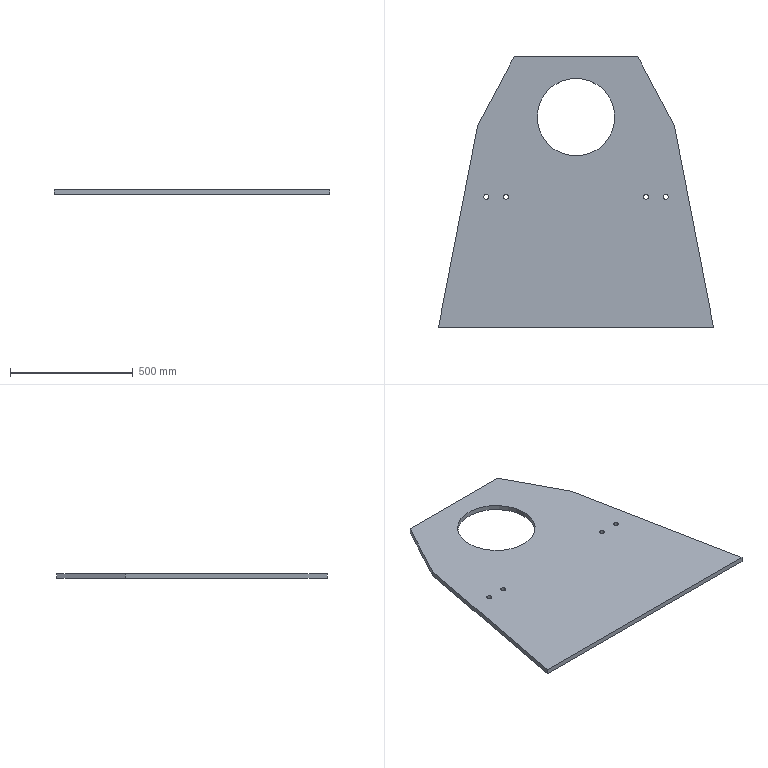Part | SolidWorks | features BaseBody 1 | 1 solid | 18 faces | box 1120 x 1100 x 20 mm | volume 17817233 mm3 | cylinder 10 | plane 8 | commonest cylinder face diameters 20 x8 316 x2
STEP:
#1=CARTESIAN_POINT('',(4376.449,1438.717,20.));
#2=VERTEX_POINT('',#1);
#3=CARTESIAN_POINT('',(4396.449,1438.717,20.));
#4=VERTEX_POINT('',#3);
#5=CARTESIAN_POINT('',(4386.449,1438.717,20.));
#6=DIRECTION('',(0.,0.,1.));
#7=DIRECTION('',(1.,0.,0.));
#8=AXIS2_PLACEMENT_3D('',#5,#6,#7);
#9=CIRCLE('',#8,10.);
#10=EDGE_CURVE('',#2,#4,#9,.T.);
#11=ORIENTED_EDGE('',*,*,#10,.T.);
#12=CARTESIAN_POINT('',(4396.449,1438.717,0.));
#13=VERTEX_POINT('',#12);
#14=CARTESIAN_POINT('',(4396.449,1438.717,20.));
#15=DIRECTION('',(0.,0.,-1.));
#16=VECTOR('',#15,1000.);
#17=LINE('',#14,#16);
#18=EDGE_CURVE('',#4,#13,#17,.T.);
#19=ORIENTED_EDGE('',*,*,#18,.T.);
#20=CARTESIAN_POINT('',(4376.449,1438.717,0.));
#21=VERTEX_POINT('',#20);
#22=CARTESIAN_POINT('',(4386.449,1438.717,0.));
#23=DIRECTION('',(0.,0.,1.));
#24=DIRECTION('',(1.,0.,0.));
#25=AXIS2_PLACEMENT_3D('',#22,#23,#24);
#26=CIRCLE('',#25,10.);
#27=EDGE_CURVE('',#21,#13,#26,.T.);
#28=ORIENTED_EDGE('',*,*,#27,.F.);
#29=CARTESIAN_POINT('',(4376.449,1438.717,20.));
#30=DIRECTION('',(0.,0.,-1.));
#31=VECTOR('',#30,1000.);
#32=LINE('',#29,#31);
#33=EDGE_CURVE('',#2,#21,#32,.T.);
#34=ORIENTED_EDGE('',*,*,#33,.F.);
#35=EDGE_LOOP('',(#11,#19,#28,#34));
#36=FACE_OUTER_BOUND('',#35,.T.);
#37=CARTESIAN_POINT('',(4386.449,1438.717,20.));
#38=DIRECTION('',(0.,0.,-1.));
#39=DIRECTION('',(-1.,0.,0.));
#40=AXIS2_PLACEMENT_3D('',#37,#38,#39);
#41=CYLINDRICAL_SURFACE('',#40,10.);
#42=ADVANCED_FACE('',(#36),#41,.F.);
#43=CARTESIAN_POINT('',(4456.449,1438.717,20.));
#44=VERTEX_POINT('',#43);
#45=CARTESIAN_POINT('',(4476.449,1438.717,20.));
#46=VERTEX_POINT('',#45);
#47=CARTESIAN_POINT('',(4466.449,1438.717,20.));
#48=DIRECTION('',(0.,0.,1.));
#49=DIRECTION('',(1.,0.,0.));
#50=AXIS2_PLACEMENT_3D('',#47,#48,#49);
#51=CIRCLE('',#50,10.);
#52=EDGE_CURVE('',#44,#46,#51,.T.);
#53=ORIENTED_EDGE('',*,*,#52,.T.);
#54=CARTESIAN_POINT('',(4476.449,1438.717,0.));
#55=VERTEX_POINT('',#54);
#56=CARTESIAN_POINT('',(4476.449,1438.717,20.));
#57=DIRECTION('',(0.,0.,-1.));
#58=VECTOR('',#57,1000.);
#59=LINE('',#56,#58);
#60=EDGE_CURVE('',#46,#55,#59,.T.);
#61=ORIENTED_EDGE('',*,*,#60,.T.);
#62=CARTESIAN_POINT('',(4456.449,1438.717,0.));
#63=VERTEX_POINT('',#62);
#64=CARTESIAN_POINT('',(4466.449,1438.717,0.));
#65=DIRECTION('',(0.,0.,1.));
#66=DIRECTION('',(1.,0.,0.));
#67=AXIS2_PLACEMENT_3D('',#64,#65,#66);
#68=CIRCLE('',#67,10.);
#69=EDGE_CURVE('',#63,#55,#68,.T.);
#70=ORIENTED_EDGE('',*,*,#69,.F.);
#71=CARTESIAN_POINT('',(4456.449,1438.717,20.));
#72=DIRECTION('',(0.,0.,-1.));
#73=VECTOR('',#72,1000.);
#74=LINE('',#71,#73);
#75=EDGE_CURVE('',#44,#63,#74,.T.);
#76=ORIENTED_EDGE('',*,*,#75,.F.);
#77=EDGE_LOOP('',(#53,#61,#70,#76));
#78=FACE_OUTER_BOUND('',#77,.T.);
#79=CARTESIAN_POINT('',(4466.449,1438.717,20.));
#80=DIRECTION('',(0.,0.,-1.));
#81=DIRECTION('',(-1.,0.,0.));
#82=AXIS2_PLACEMENT_3D('',#79,#80,#81);
#83=CYLINDRICAL_SURFACE('',#82,10.);
#84=ADVANCED_FACE('',(#78),#83,.F.);
#85=CARTESIAN_POINT('',(4593.449,1763.717,20.));
#86=VERTEX_POINT('',#85);
#87=CARTESIAN_POINT('',(4909.449,1763.717,20.));
#88=VERTEX_POINT('',#87);
#89=CARTESIAN_POINT('',(4751.449,1763.717,20.));
#90=DIRECTION('',(0.,0.,1.));
#91=DIRECTION('',(1.,0.,0.));
#92=AXIS2_PLACEMENT_3D('',#89,#90,#91);
#93=CIRCLE('',#92,158.);
#94=EDGE_CURVE('',#86,#88,#93,.T.);
#95=ORIENTED_EDGE('',*,*,#94,.T.);
#96=CARTESIAN_POINT('',(4909.449,1763.717,0.));
#97=VERTEX_POINT('',#96);
#98=CARTESIAN_POINT('',(4909.449,1763.717,20.));
#99=DIRECTION('',(0.,0.,-1.));
#100=VECTOR('',#99,1000.);
#101=LINE('',#98,#100);
#102=EDGE_CURVE('',#88,#97,#101,.T.);
#103=ORIENTED_EDGE('',*,*,#102,.T.);
#104=CARTESIAN_POINT('',(4593.449,1763.717,0.));
#105=VERTEX_POINT('',#104);
#106=CARTESIAN_POINT('',(4751.449,1763.717,0.));
#107=DIRECTION('',(0.,0.,1.));
#108=DIRECTION('',(1.,0.,0.));
#109=AXIS2_PLACEMENT_3D('',#106,#107,#108);
#110=CIRCLE('',#109,158.);
#111=EDGE_CURVE('',#105,#97,#110,.T.);
#112=ORIENTED_EDGE('',*,*,#111,.F.);
#113=CARTESIAN_POINT('',(4593.449,1763.717,20.));
#114=DIRECTION('',(0.,0.,-1.));
#115=VECTOR('',#114,1000.);
#116=LINE('',#113,#115);
#117=EDGE_CURVE('',#86,#105,#116,.T.);
#118=ORIENTED_EDGE('',*,*,#117,.F.);
#119=EDGE_LOOP('',(#95,#103,#112,#118));
#120=FACE_OUTER_BOUND('',#119,.T.);
#121=CARTESIAN_POINT('',(4751.449,1763.717,20.));
#122=DIRECTION('',(0.,0.,-1.));
#123=DIRECTION('',(-1.,0.,0.));
#124=AXIS2_PLACEMENT_3D('',#121,#122,#123);
#125=CYLINDRICAL_SURFACE('',#124,158.);
#126=ADVANCED_FACE('',(#120),#125,.F.);
#127=CARTESIAN_POINT('',(5106.449,1438.717,20.));
#128=VERTEX_POINT('',#127);
#129=CARTESIAN_POINT('',(5126.449,1438.717,20.));
#130=VERTEX_POINT('',#129);
#131=CARTESIAN_POINT('',(5116.449,1438.717,20.));
#132=DIRECTION('',(0.,0.,1.));
#133=DIRECTION('',(1.,0.,0.));
#134=AXIS2_PLACEMENT_3D('',#131,#132,#133);
#135=CIRCLE('',#134,10.);
#136=EDGE_CURVE('',#128,#130,#135,.T.);
#137=ORIENTED_EDGE('',*,*,#136,.T.);
#138=CARTESIAN_POINT('',(5126.449,1438.717,0.));
#139=VERTEX_POINT('',#138);
#140=CARTESIAN_POINT('',(5126.449,1438.717,20.));
#141=DIRECTION('',(0.,0.,-1.));
#142=VECTOR('',#141,1000.);
#143=LINE('',#140,#142);
#144=EDGE_CURVE('',#130,#139,#143,.T.);
#145=ORIENTED_EDGE('',*,*,#144,.T.);
#146=CARTESIAN_POINT('',(5106.449,1438.717,0.));
#147=VERTEX_POINT('',#146);
#148=CARTESIAN_POINT('',(5116.449,1438.717,0.));
#149=DIRECTION('',(0.,0.,1.));
#150=DIRECTION('',(1.,0.,0.));
#151=AXIS2_PLACEMENT_3D('',#148,#149,#150);
#152=CIRCLE('',#151,10.);
#153=EDGE_CURVE('',#147,#139,#152,.T.);
#154=ORIENTED_EDGE('',*,*,#153,.F.);
#155=CARTESIAN_POINT('',(5106.449,1438.717,20.));
#156=DIRECTION('',(0.,0.,-1.));
#157=VECTOR('',#156,1000.);
#158=LINE('',#155,#157);
#159=EDGE_CURVE('',#128,#147,#158,.T.);
#160=ORIENTED_EDGE('',*,*,#159,.F.);
#161=EDGE_LOOP('',(#137,#145,#154,#160));
#162=FACE_OUTER_BOUND('',#161,.T.);
#163=CARTESIAN_POINT('',(5116.449,1438.717,20.));
#164=DIRECTION('',(0.,0.,-1.));
#165=DIRECTION('',(-1.,0.,0.));
#166=AXIS2_PLACEMENT_3D('',#163,#164,#165);
#167=CYLINDRICAL_SURFACE('',#166,10.);
#168=ADVANCED_FACE('',(#162),#167,.F.);
#169=CARTESIAN_POINT('',(5026.449,1438.717,20.));
#170=VERTEX_POINT('',#169);
#171=CARTESIAN_POINT('',(5046.449,1438.717,20.));
#172=VERTEX_POINT('',#171);
#173=CARTESIAN_POINT('',(5036.449,1438.717,20.));
#174=DIRECTION('',(0.,0.,1.));
#175=DIRECTION('',(1.,0.,0.));
#176=AXIS2_PLACEMENT_3D('',#173,#174,#175);
#177=CIRCLE('',#176,10.);
#178=EDGE_CURVE('',#170,#172,#177,.T.);
#179=ORIENTED_EDGE('',*,*,#178,.T.);
#180=CARTESIAN_POINT('',(5046.449,1438.717,0.));
#181=VERTEX_POINT('',#180);
#182=CARTESIAN_POINT('',(5046.449,1438.717,20.));
#183=DIRECTION('',(0.,0.,-1.));
#184=VECTOR('',#183,1000.);
#185=LINE('',#182,#184);
#186=EDGE_CURVE('',#172,#181,#185,.T.);
#187=ORIENTED_EDGE('',*,*,#186,.T.);
#188=CARTESIAN_POINT('',(5026.449,1438.717,0.));
#189=VERTEX_POINT('',#188);
#190=CARTESIAN_POINT('',(5036.449,1438.717,0.));
#191=DIRECTION('',(0.,0.,1.));
#192=DIRECTION('',(1.,0.,0.));
#193=AXIS2_PLACEMENT_3D('',#190,#191,#192);
#194=CIRCLE('',#193,10.);
#195=EDGE_CURVE('',#189,#181,#194,.T.);
#196=ORIENTED_EDGE('',*,*,#195,.F.);
#197=CARTESIAN_POINT('',(5026.449,1438.717,20.));
#198=DIRECTION('',(0.,0.,-1.));
#199=VECTOR('',#198,1000.);
#200=LINE('',#197,#199);
#201=EDGE_CURVE('',#170,#189,#200,.T.);
#202=ORIENTED_EDGE('',*,*,#201,.F.);
#203=EDGE_LOOP('',(#179,#187,#196,#202));
#204=FACE_OUTER_BOUND('',#203,.T.);
#205=CARTESIAN_POINT('',(5036.449,1438.717,20.));
#206=DIRECTION('',(0.,0.,-1.));
#207=DIRECTION('',(-1.,0.,0.));
#208=AXIS2_PLACEMENT_3D('',#205,#206,#207);
#209=CYLINDRICAL_SURFACE('',#208,10.);
#210=ADVANCED_FACE('',(#204),#209,.F.);
#211=ORIENTED_EDGE('',*,*,#52,.F.);
#212=CARTESIAN_POINT('',(4466.449,1438.717,20.));
#213=DIRECTION('',(0.,0.,1.));
#214=DIRECTION('',(1.,0.,0.));
#215=AXIS2_PLACEMENT_3D('',#212,#213,#214);
#216=CIRCLE('',#215,10.);
#217=EDGE_CURVE('',#46,#44,#216,.T.);
#218=ORIENTED_EDGE('',*,*,#217,.F.);
#219=EDGE_LOOP('',(#211,#218));
#220=FACE_BOUND('',#219,.T.);
#221=ORIENTED_EDGE('',*,*,#136,.F.);
#222=CARTESIAN_POINT('',(5116.449,1438.717,20.));
#223=DIRECTION('',(0.,0.,1.));
#224=DIRECTION('',(1.,0.,0.));
#225=AXIS2_PLACEMENT_3D('',#222,#223,#224);
#226=CIRCLE('',#225,10.);
#227=EDGE_CURVE('',#130,#128,#226,.T.);
#228=ORIENTED_EDGE('',*,*,#227,.F.);
#229=EDGE_LOOP('',(#221,#228));
#230=FACE_BOUND('',#229,.T.);
#231=CARTESIAN_POINT('',(4351.039,1729.734,20.));
#232=VERTEX_POINT('',#231);
#233=CARTESIAN_POINT('',(4191.449,908.717,20.));
#234=VERTEX_POINT('',#233);
#235=CARTESIAN_POINT('',(4351.039,1729.734,20.));
#236=DIRECTION('',(-0.1908,-0.9816,0.));
#237=VECTOR('',#236,1000.);
#238=LINE('',#235,#237);
#239=EDGE_CURVE('',#232,#234,#238,.T.);
#240=ORIENTED_EDGE('',*,*,#239,.T.);
#241=CARTESIAN_POINT('',(5311.449,908.717,20.));
#242=VERTEX_POINT('',#241);
#243=CARTESIAN_POINT('',(4191.449,908.717,20.));
#244=DIRECTION('',(1.,0.,0.));
#245=VECTOR('',#244,1000.);
#246=LINE('',#243,#245);
#247=EDGE_CURVE('',#234,#242,#246,.T.);
#248=ORIENTED_EDGE('',*,*,#247,.T.);
#249=CARTESIAN_POINT('',(5151.86,1729.734,20.));
#250=VERTEX_POINT('',#249);
#251=CARTESIAN_POINT('',(5151.86,1729.734,20.));
#252=DIRECTION('',(-0.1908,0.9816,0.));
#253=VECTOR('',#252,1000.);
#254=LINE('',#251,#253);
#255=EDGE_CURVE('',#242,#250,#254,.T.);
#256=ORIENTED_EDGE('',*,*,#255,.T.);
#257=CARTESIAN_POINT('',(5003.522,2008.717,20.));
#258=VERTEX_POINT('',#257);
#259=CARTESIAN_POINT('',(5003.522,2008.717,20.));
#260=DIRECTION('',(-0.4695,0.8829,0.));
#261=VECTOR('',#260,1000.);
#262=LINE('',#259,#261);
#263=EDGE_CURVE('',#250,#258,#262,.T.);
#264=ORIENTED_EDGE('',*,*,#263,.T.);
#265=CARTESIAN_POINT('',(4499.377,2008.717,20.));
#266=VERTEX_POINT('',#265);
#267=CARTESIAN_POINT('',(4499.377,2008.717,20.));
#268=DIRECTION('',(-1.,0.,0.));
#269=VECTOR('',#268,1000.);
#270=LINE('',#267,#269);
#271=EDGE_CURVE('',#258,#266,#270,.T.);
#272=ORIENTED_EDGE('',*,*,#271,.T.);
#273=CARTESIAN_POINT('',(4499.377,2008.717,20.));
#274=DIRECTION('',(-0.4695,-0.8829,0.));
#275=VECTOR('',#274,1000.);
#276=LINE('',#273,#275);
#277=EDGE_CURVE('',#266,#232,#276,.T.);
#278=ORIENTED_EDGE('',*,*,#277,.T.);
#279=EDGE_LOOP('',(#240,#248,#256,#264,#272,#278));
#280=FACE_OUTER_BOUND('',#279,.T.);
#281=ORIENTED_EDGE('',*,*,#178,.F.);
#282=CARTESIAN_POINT('',(5036.449,1438.717,20.));
#283=DIRECTION('',(0.,0.,1.));
#284=DIRECTION('',(1.,0.,0.));
#285=AXIS2_PLACEMENT_3D('',#282,#283,#284);
#286=CIRCLE('',#285,10.);
#287=EDGE_CURVE('',#172,#170,#286,.T.);
#288=ORIENTED_EDGE('',*,*,#287,.F.);
#289=EDGE_LOOP('',(#281,#288));
#290=FACE_BOUND('',#289,.T.);
#291=ORIENTED_EDGE('',*,*,#94,.F.);
#292=CARTESIAN_POINT('',(4751.449,1763.717,20.));
#293=DIRECTION('',(0.,0.,1.));
#294=DIRECTION('',(1.,0.,0.));
#295=AXIS2_PLACEMENT_3D('',#292,#293,#294);
#296=CIRCLE('',#295,158.);
#297=EDGE_CURVE('',#88,#86,#296,.T.);
#298=ORIENTED_EDGE('',*,*,#297,.F.);
#299=EDGE_LOOP('',(#291,#298));
#300=FACE_BOUND('',#299,.T.);
#301=ORIENTED_EDGE('',*,*,#10,.F.);
#302=CARTESIAN_POINT('',(4386.449,1438.717,20.));
#303=DIRECTION('',(0.,0.,1.));
#304=DIRECTION('',(1.,0.,0.));
#305=AXIS2_PLACEMENT_3D('',#302,#303,#304);
#306=CIRCLE('',#305,10.);
#307=EDGE_CURVE('',#4,#2,#306,.T.);
#308=ORIENTED_EDGE('',*,*,#307,.F.);
#309=EDGE_LOOP('',(#301,#308));
#310=FACE_BOUND('',#309,.T.);
#311=CARTESIAN_POINT('',(0.,0.,20.));
#312=DIRECTION('',(0.,0.,1.));
#313=DIRECTION('',(1.,0.,0.));
#314=AXIS2_PLACEMENT_3D('',#311,#312,#313);
#315=PLANE('',#314);
#316=ADVANCED_FACE('',(#220,#230,#280,#290,#300,#310),#315,.T.);
#317=CARTESIAN_POINT('',(4351.039,1729.734,0.));
#318=VERTEX_POINT('',#317);
#319=CARTESIAN_POINT('',(4191.449,908.717,0.));
#320=VERTEX_POINT('',#319);
#321=CARTESIAN_POINT('',(4351.039,1729.734,0.));
#322=DIRECTION('',(-0.1908,-0.9816,0.));
#323=VECTOR('',#322,1000.);
#324=LINE('',#321,#323);
#325=EDGE_CURVE('',#318,#320,#324,.T.);
#326=ORIENTED_EDGE('',*,*,#325,.F.);
#327=CARTESIAN_POINT('',(4499.377,2008.717,0.));
#328=VERTEX_POINT('',#327);
#329=CARTESIAN_POINT('',(4499.377,2008.717,0.));
#330=DIRECTION('',(-0.4695,-0.8829,0.));
#331=VECTOR('',#330,1000.);
#332=LINE('',#329,#331);
#333=EDGE_CURVE('',#328,#318,#332,.T.);
#334=ORIENTED_EDGE('',*,*,#333,.F.);
#335=CARTESIAN_POINT('',(5003.522,2008.717,0.));
#336=VERTEX_POINT('',#335);
#337=CARTESIAN_POINT('',(4499.377,2008.717,0.));
#338=DIRECTION('',(-1.,0.,0.));
#339=VECTOR('',#338,1000.);
#340=LINE('',#337,#339);
#341=EDGE_CURVE('',#336,#328,#340,.T.);
#342=ORIENTED_EDGE('',*,*,#341,.F.);
#343=CARTESIAN_POINT('',(5151.86,1729.734,0.));
#344=VERTEX_POINT('',#343);
#345=CARTESIAN_POINT('',(5003.522,2008.717,0.));
#346=DIRECTION('',(-0.4695,0.8829,0.));
#347=VECTOR('',#346,1000.);
#348=LINE('',#345,#347);
#349=EDGE_CURVE('',#344,#336,#348,.T.);
#350=ORIENTED_EDGE('',*,*,#349,.F.);
#351=CARTESIAN_POINT('',(5311.449,908.717,0.));
#352=VERTEX_POINT('',#351);
#353=CARTESIAN_POINT('',(5151.86,1729.734,0.));
#354=DIRECTION('',(-0.1908,0.9816,0.));
#355=VECTOR('',#354,1000.);
#356=LINE('',#353,#355);
#357=EDGE_CURVE('',#352,#344,#356,.T.);
#358=ORIENTED_EDGE('',*,*,#357,.F.);
#359=CARTESIAN_POINT('',(4191.449,908.717,0.));
#360=DIRECTION('',(1.,0.,0.));
#361=VECTOR('',#360,1000.);
#362=LINE('',#359,#361);
#363=EDGE_CURVE('',#320,#352,#362,.T.);
#364=ORIENTED_EDGE('',*,*,#363,.F.);
#365=EDGE_LOOP('',(#326,#334,#342,#350,#358,#364));
#366=FACE_OUTER_BOUND('',#365,.T.);
#367=ORIENTED_EDGE('',*,*,#195,.T.);
#368=CARTESIAN_POINT('',(5036.449,1438.717,0.));
#369=DIRECTION('',(0.,0.,1.));
#370=DIRECTION('',(1.,0.,0.));
#371=AXIS2_PLACEMENT_3D('',#368,#369,#370);
#372=CIRCLE('',#371,10.);
#373=EDGE_CURVE('',#181,#189,#372,.T.);
#374=ORIENTED_EDGE('',*,*,#373,.T.);
#375=EDGE_LOOP('',(#367,#374));
#376=FACE_BOUND('',#375,.T.);
#377=ORIENTED_EDGE('',*,*,#153,.T.);
#378=CARTESIAN_POINT('',(5116.449,1438.717,0.));
#379=DIRECTION('',(0.,0.,1.));
#380=DIRECTION('',(1.,0.,0.));
#381=AXIS2_PLACEMENT_3D('',#378,#379,#380);
#382=CIRCLE('',#381,10.);
#383=EDGE_CURVE('',#139,#147,#382,.T.);
#384=ORIENTED_EDGE('',*,*,#383,.T.);
#385=EDGE_LOOP('',(#377,#384));
#386=FACE_BOUND('',#385,.T.);
#387=ORIENTED_EDGE('',*,*,#111,.T.);
#388=CARTESIAN_POINT('',(4751.449,1763.717,0.));
#389=DIRECTION('',(0.,0.,1.));
#390=DIRECTION('',(1.,0.,0.));
#391=AXIS2_PLACEMENT_3D('',#388,#389,#390);
#392=CIRCLE('',#391,158.);
#393=EDGE_CURVE('',#97,#105,#392,.T.);
#394=ORIENTED_EDGE('',*,*,#393,.T.);
#395=EDGE_LOOP('',(#387,#394));
#396=FACE_BOUND('',#395,.T.);
#397=ORIENTED_EDGE('',*,*,#69,.T.);
#398=CARTESIAN_POINT('',(4466.449,1438.717,0.));
#399=DIRECTION('',(0.,0.,1.));
#400=DIRECTION('',(1.,0.,0.));
#401=AXIS2_PLACEMENT_3D('',#398,#399,#400);
#402=CIRCLE('',#401,10.);
#403=EDGE_CURVE('',#55,#63,#402,.T.);
#404=ORIENTED_EDGE('',*,*,#403,.T.);
#405=EDGE_LOOP('',(#397,#404));
#406=FACE_BOUND('',#405,.T.);
#407=ORIENTED_EDGE('',*,*,#27,.T.);
#408=CARTESIAN_POINT('',(4386.449,1438.717,0.));
#409=DIRECTION('',(0.,0.,1.));
#410=DIRECTION('',(1.,0.,0.));
#411=AXIS2_PLACEMENT_3D('',#408,#409,#410);
#412=CIRCLE('',#411,10.);
#413=EDGE_CURVE('',#13,#21,#412,.T.);
#414=ORIENTED_EDGE('',*,*,#413,.T.);
#415=EDGE_LOOP('',(#407,#414));
#416=FACE_BOUND('',#415,.T.);
#417=CARTESIAN_POINT('',(0.,0.,0.));
#418=DIRECTION('',(0.,0.,1.));
#419=DIRECTION('',(1.,0.,0.));
#420=AXIS2_PLACEMENT_3D('',#417,#418,#419);
#421=PLANE('',#420);
#422=ADVANCED_FACE('',(#366,#376,#386,#396,#406,#416),#421,.F.);
#423=ORIENTED_EDGE('',*,*,#325,.T.);
#424=CARTESIAN_POINT('',(4191.449,908.717,20.));
#425=DIRECTION('',(0.,0.,-1.));
#426=VECTOR('',#425,1000.);
#427=LINE('',#424,#426);
#428=EDGE_CURVE('',#234,#320,#427,.T.);
#429=ORIENTED_EDGE('',*,*,#428,.F.);
#430=ORIENTED_EDGE('',*,*,#239,.F.);
#431=CARTESIAN_POINT('',(4351.039,1729.734,20.));
#432=DIRECTION('',(0.,0.,-1.));
#433=VECTOR('',#432,1000.);
#434=LINE('',#431,#433);
#435=EDGE_CURVE('',#232,#318,#434,.T.);
#436=ORIENTED_EDGE('',*,*,#435,.T.);
#437=EDGE_LOOP('',(#423,#429,#430,#436));
#438=FACE_OUTER_BOUND('',#437,.T.);
#439=CARTESIAN_POINT('',(4351.039,1729.734,20.));
#440=DIRECTION('',(0.9816,-0.1908,0.));
#441=DIRECTION('',(0.1908,0.9816,0.));
#442=AXIS2_PLACEMENT_3D('',#439,#440,#441);
#443=PLANE('',#442);
#444=ADVANCED_FACE('',(#438),#443,.F.);
#445=ORIENTED_EDGE('',*,*,#363,.T.);
#446=CARTESIAN_POINT('',(5311.449,908.717,20.));
#447=DIRECTION('',(0.,0.,-1.));
#448=VECTOR('',#447,1000.);
#449=LINE('',#446,#448);
#450=EDGE_CURVE('',#242,#352,#449,.T.);
#451=ORIENTED_EDGE('',*,*,#450,.F.);
#452=ORIENTED_EDGE('',*,*,#247,.F.);
#453=ORIENTED_EDGE('',*,*,#428,.T.);
#454=EDGE_LOOP('',(#445,#451,#452,#453));
#455=FACE_OUTER_BOUND('',#454,.T.);
#456=CARTESIAN_POINT('',(4191.449,908.717,20.));
#457=DIRECTION('',(0.,1.,0.));
#458=DIRECTION('',(0.,0.,1.));
#459=AXIS2_PLACEMENT_3D('',#456,#457,#458);
#460=PLANE('',#459);
#461=ADVANCED_FACE('',(#455),#460,.F.);
#462=ORIENTED_EDGE('',*,*,#357,.T.);
#463=CARTESIAN_POINT('',(5151.86,1729.734,20.));
#464=DIRECTION('',(0.,0.,-1.));
#465=VECTOR('',#464,1000.);
#466=LINE('',#463,#465);
#467=EDGE_CURVE('',#250,#344,#466,.T.);
#468=ORIENTED_EDGE('',*,*,#467,.F.);
#469=ORIENTED_EDGE('',*,*,#255,.F.);
#470=ORIENTED_EDGE('',*,*,#450,.T.);
#471=EDGE_LOOP('',(#462,#468,#469,#470));
#472=FACE_OUTER_BOUND('',#471,.T.);
#473=CARTESIAN_POINT('',(5151.86,1729.734,20.));
#474=DIRECTION('',(-0.9816,-0.1908,0.));
#475=DIRECTION('',(0.1908,-0.9816,0.));
#476=AXIS2_PLACEMENT_3D('',#473,#474,#475);
#477=PLANE('',#476);
#478=ADVANCED_FACE('',(#472),#477,.F.);
#479=ORIENTED_EDGE('',*,*,#349,.T.);
#480=CARTESIAN_POINT('',(5003.522,2008.717,20.));
#481=DIRECTION('',(0.,0.,-1.));
#482=VECTOR('',#481,1000.);
#483=LINE('',#480,#482);
#484=EDGE_CURVE('',#258,#336,#483,.T.);
#485=ORIENTED_EDGE('',*,*,#484,.F.);
#486=ORIENTED_EDGE('',*,*,#263,.F.);
#487=ORIENTED_EDGE('',*,*,#467,.T.);
#488=EDGE_LOOP('',(#479,#485,#486,#487));
#489=FACE_OUTER_BOUND('',#488,.T.);
#490=CARTESIAN_POINT('',(5003.522,2008.717,20.));
#491=DIRECTION('',(-0.8829,-0.4695,0.));
#492=DIRECTION('',(0.4695,-0.8829,0.));
#493=AXIS2_PLACEMENT_3D('',#490,#491,#492);
#494=PLANE('',#493);
#495=ADVANCED_FACE('',(#489),#494,.F.);
#496=ORIENTED_EDGE('',*,*,#341,.T.);
#497=CARTESIAN_POINT('',(4499.377,2008.717,20.));
#498=DIRECTION('',(0.,0.,-1.));
#499=VECTOR('',#498,1000.);
#500=LINE('',#497,#499);
#501=EDGE_CURVE('',#266,#328,#500,.T.);
#502=ORIENTED_EDGE('',*,*,#501,.F.);
#503=ORIENTED_EDGE('',*,*,#271,.F.);
#504=ORIENTED_EDGE('',*,*,#484,.T.);
#505=EDGE_LOOP('',(#496,#502,#503,#504));
#506=FACE_OUTER_BOUND('',#505,.T.);
#507=CARTESIAN_POINT('',(4499.377,2008.717,20.));
#508=DIRECTION('',(0.,-1.,0.));
#509=DIRECTION('',(0.,0.,-1.));
#510=AXIS2_PLACEMENT_3D('',#507,#508,#509);
#511=PLANE('',#510);
#512=ADVANCED_FACE('',(#506),#511,.F.);
#513=ORIENTED_EDGE('',*,*,#333,.T.);
#514=ORIENTED_EDGE('',*,*,#435,.F.);
#515=ORIENTED_EDGE('',*,*,#277,.F.);
#516=ORIENTED_EDGE('',*,*,#501,.T.);
#517=EDGE_LOOP('',(#513,#514,#515,#516));
#518=FACE_OUTER_BOUND('',#517,.T.);
#519=CARTESIAN_POINT('',(4499.377,2008.717,20.));
#520=DIRECTION('',(0.8829,-0.4695,0.));
#521=DIRECTION('',(0.4695,0.8829,0.));
#522=AXIS2_PLACEMENT_3D('',#519,#520,#521);
#523=PLANE('',#522);
#524=ADVANCED_FACE('',(#518),#523,.F.);
#525=ORIENTED_EDGE('',*,*,#186,.F.);
#526=ORIENTED_EDGE('',*,*,#287,.T.);
#527=ORIENTED_EDGE('',*,*,#201,.T.);
#528=ORIENTED_EDGE('',*,*,#373,.F.);
#529=EDGE_LOOP('',(#525,#526,#527,#528));
#530=FACE_OUTER_BOUND('',#529,.T.);
#531=CARTESIAN_POINT('',(5036.449,1438.717,20.));
#532=DIRECTION('',(0.,0.,-1.));
#533=DIRECTION('',(-1.,0.,0.));
#534=AXIS2_PLACEMENT_3D('',#531,#532,#533);
#535=CYLINDRICAL_SURFACE('',#534,10.);
#536=ADVANCED_FACE('',(#530),#535,.F.);
#537=ORIENTED_EDGE('',*,*,#144,.F.);
#538=ORIENTED_EDGE('',*,*,#227,.T.);
#539=ORIENTED_EDGE('',*,*,#159,.T.);
#540=ORIENTED_EDGE('',*,*,#383,.F.);
#541=EDGE_LOOP('',(#537,#538,#539,#540));
#542=FACE_OUTER_BOUND('',#541,.T.);
#543=CARTESIAN_POINT('',(5116.449,1438.717,20.));
#544=DIRECTION('',(0.,0.,-1.));
#545=DIRECTION('',(-1.,0.,0.));
#546=AXIS2_PLACEMENT_3D('',#543,#544,#545);
#547=CYLINDRICAL_SURFACE('',#546,10.);
#548=ADVANCED_FACE('',(#542),#547,.F.);
#549=ORIENTED_EDGE('',*,*,#102,.F.);
#550=ORIENTED_EDGE('',*,*,#297,.T.);
#551=ORIENTED_EDGE('',*,*,#117,.T.);
#552=ORIENTED_EDGE('',*,*,#393,.F.);
#553=EDGE_LOOP('',(#549,#550,#551,#552));
#554=FACE_OUTER_BOUND('',#553,.T.);
#555=CARTESIAN_POINT('',(4751.449,1763.717,20.));
#556=DIRECTION('',(0.,0.,-1.));
#557=DIRECTION('',(-1.,0.,0.));
#558=AXIS2_PLACEMENT_3D('',#555,#556,#557);
#559=CYLINDRICAL_SURFACE('',#558,158.);
#560=ADVANCED_FACE('',(#554),#559,.F.);
#561=ORIENTED_EDGE('',*,*,#60,.F.);
#562=ORIENTED_EDGE('',*,*,#217,.T.);
#563=ORIENTED_EDGE('',*,*,#75,.T.);
#564=ORIENTED_EDGE('',*,*,#403,.F.);
#565=EDGE_LOOP('',(#561,#562,#563,#564));
#566=FACE_OUTER_BOUND('',#565,.T.);
#567=CARTESIAN_POINT('',(4466.449,1438.717,20.));
#568=DIRECTION('',(0.,0.,-1.));
#569=DIRECTION('',(-1.,0.,0.));
#570=AXIS2_PLACEMENT_3D('',#567,#568,#569);
#571=CYLINDRICAL_SURFACE('',#570,10.);
#572=ADVANCED_FACE('',(#566),#571,.F.);
#573=ORIENTED_EDGE('',*,*,#18,.F.);
#574=ORIENTED_EDGE('',*,*,#307,.T.);
#575=ORIENTED_EDGE('',*,*,#33,.T.);
#576=ORIENTED_EDGE('',*,*,#413,.F.);
#577=EDGE_LOOP('',(#573,#574,#575,#576));
#578=FACE_OUTER_BOUND('',#577,.T.);
#579=CARTESIAN_POINT('',(4386.449,1438.717,20.));
#580=DIRECTION('',(0.,0.,-1.));
#581=DIRECTION('',(-1.,0.,0.));
#582=AXIS2_PLACEMENT_3D('',#579,#580,#581);
#583=CYLINDRICAL_SURFACE('',#582,10.);
#584=ADVANCED_FACE('',(#578),#583,.F.);
#585=CLOSED_SHELL('',(#42,#84,#126,#168,#210,#316,#422,#444,#461,#478,#495,#512,#524,#536,#548,#560,#572,#584));
#586=MANIFOLD_SOLID_BREP('',#585);
#587=CARTESIAN_POINT('',(0.,0.,0.));
#588=DIRECTION('',(0.,0.,1.));
#589=DIRECTION('',(1.,0.,0.));
#590=AXIS2_PLACEMENT_3D('',#587,#588,#589);
#591=(LENGTH_UNIT()NAMED_UNIT(*)SI_UNIT(.MILLI.,.METRE.));
#592=UNCERTAINTY_MEASURE_WITH_UNIT(LENGTH_MEASURE(0.00001),#591,'','');
#593=(NAMED_UNIT(*)PLANE_ANGLE_UNIT()SI_UNIT($,.RADIAN.));
#594=(NAMED_UNIT(*)SI_UNIT($,.STERADIAN.)SOLID_ANGLE_UNIT());
#595=(GEOMETRIC_REPRESENTATION_CONTEXT(3)GLOBAL_UNCERTAINTY_ASSIGNED_CONTEXT((#592))GLOBAL_UNIT_ASSIGNED_CONTEXT((#591,#593,#594))REPRESENTATION_CONTEXT('',''));
#596=ADVANCED_BREP_SHAPE_REPRESENTATION('',(#586,#590),#595);